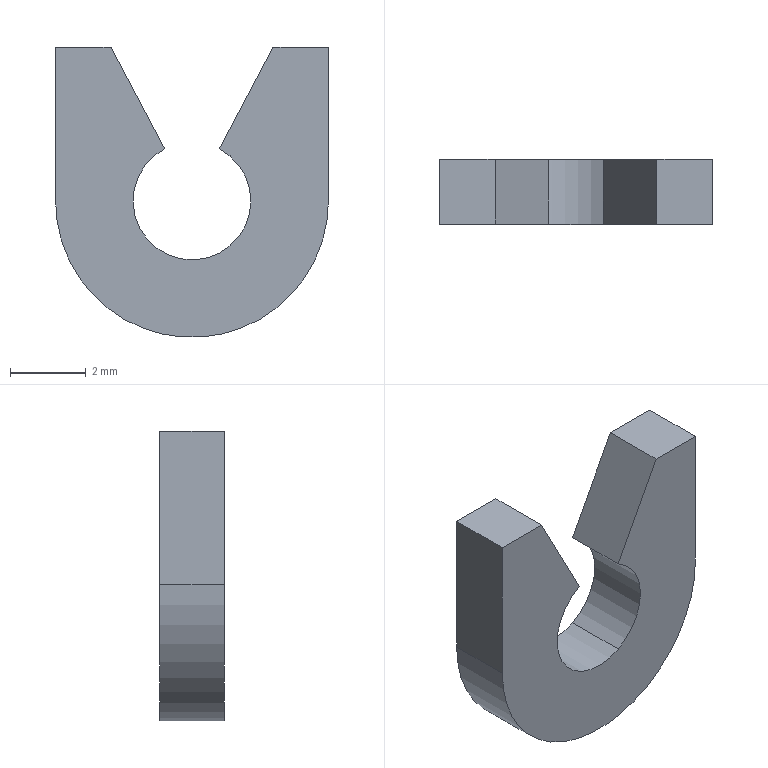Part | SolidWorks | features BaseBody 1 | 1 solid | 11 faces | box 7.18 x 1.7 x 7.64 mm | volume 58.331 mm3 | plane 8 | cylinder 3 | commonest cylinder face diameters 3.1 x2 7.18 x1
STEP:
#1=CARTESIAN_POINT('',(0.7215,1.7,1.372));
#2=VERTEX_POINT('',#1);
#3=CARTESIAN_POINT('',(0.7215,1.7,-1.372));
#4=VERTEX_POINT('',#3);
#5=CARTESIAN_POINT('',(0.,1.7,0.));
#6=DIRECTION('',(0.,1.,0.));
#7=DIRECTION('',(0.4655,0.,0.8851));
#8=AXIS2_PLACEMENT_3D('',#5,#6,#7);
#9=CIRCLE('',#8,1.55);
#10=EDGE_CURVE('',#2,#4,#9,.T.);
#11=ORIENTED_EDGE('',*,*,#10,.T.);
#12=CARTESIAN_POINT('',(0.7215,0.,-1.372));
#13=VERTEX_POINT('',#12);
#14=CARTESIAN_POINT('',(0.7215,1.7,-1.372));
#15=DIRECTION('',(0.,-1.,0.));
#16=VECTOR('',#15,1000.);
#17=LINE('',#14,#16);
#18=EDGE_CURVE('',#4,#13,#17,.T.);
#19=ORIENTED_EDGE('',*,*,#18,.T.);
#20=CARTESIAN_POINT('',(0.7215,0.,1.372));
#21=VERTEX_POINT('',#20);
#22=CARTESIAN_POINT('',(0.,0.,0.));
#23=DIRECTION('',(0.,-1.,0.));
#24=DIRECTION('',(-0.4655,0.,0.8851));
#25=AXIS2_PLACEMENT_3D('',#22,#23,#24);
#26=CIRCLE('',#25,1.55);
#27=EDGE_CURVE('',#13,#21,#26,.T.);
#28=ORIENTED_EDGE('',*,*,#27,.T.);
#29=CARTESIAN_POINT('',(0.7215,0.,1.372));
#30=DIRECTION('',(0.,1.,0.));
#31=VECTOR('',#30,1000.);
#32=LINE('',#29,#31);
#33=EDGE_CURVE('',#21,#2,#32,.T.);
#34=ORIENTED_EDGE('',*,*,#33,.T.);
#35=EDGE_LOOP('',(#11,#19,#28,#34));
#36=FACE_OUTER_BOUND('',#35,.T.);
#37=CARTESIAN_POINT('',(0.,1.7,0.));
#38=DIRECTION('',(0.,-1.,0.));
#39=DIRECTION('',(-0.4655,0.,0.8851));
#40=AXIS2_PLACEMENT_3D('',#37,#38,#39);
#41=CYLINDRICAL_SURFACE('',#40,1.55);
#42=ADVANCED_FACE('',(#36),#41,.F.);
#43=CARTESIAN_POINT('',(-3.59,0.,4.05));
#44=VERTEX_POINT('',#43);
#45=CARTESIAN_POINT('',(-2.13,0.,4.05));
#46=VERTEX_POINT('',#45);
#47=CARTESIAN_POINT('',(-3.59,0.,4.05));
#48=DIRECTION('',(1.,0.,0.));
#49=VECTOR('',#48,1000.);
#50=LINE('',#47,#49);
#51=EDGE_CURVE('',#44,#46,#50,.T.);
#52=ORIENTED_EDGE('',*,*,#51,.F.);
#53=CARTESIAN_POINT('',(-3.59,0.,0.));
#54=VERTEX_POINT('',#53);
#55=CARTESIAN_POINT('',(-3.59,0.,0.));
#56=DIRECTION('',(0.,0.,1.));
#57=VECTOR('',#56,1000.);
#58=LINE('',#55,#57);
#59=EDGE_CURVE('',#54,#44,#58,.T.);
#60=ORIENTED_EDGE('',*,*,#59,.F.);
#61=CARTESIAN_POINT('',(3.59,0.,0.));
#62=VERTEX_POINT('',#61);
#63=CARTESIAN_POINT('',(0.,0.,0.));
#64=DIRECTION('',(0.,1.,0.));
#65=DIRECTION('',(1.,0.,0.));
#66=AXIS2_PLACEMENT_3D('',#63,#64,#65);
#67=CIRCLE('',#66,3.59);
#68=EDGE_CURVE('',#62,#54,#67,.T.);
#69=ORIENTED_EDGE('',*,*,#68,.F.);
#70=CARTESIAN_POINT('',(3.59,0.,4.05));
#71=VERTEX_POINT('',#70);
#72=CARTESIAN_POINT('',(3.59,0.,4.05));
#73=DIRECTION('',(0.,0.,-1.));
#74=VECTOR('',#73,1000.);
#75=LINE('',#72,#74);
#76=EDGE_CURVE('',#71,#62,#75,.T.);
#77=ORIENTED_EDGE('',*,*,#76,.F.);
#78=CARTESIAN_POINT('',(2.13,0.,4.05));
#79=VERTEX_POINT('',#78);
#80=CARTESIAN_POINT('',(2.13,0.,4.05));
#81=DIRECTION('',(1.,0.,0.));
#82=VECTOR('',#81,1000.);
#83=LINE('',#80,#82);
#84=EDGE_CURVE('',#79,#71,#83,.T.);
#85=ORIENTED_EDGE('',*,*,#84,.F.);
#86=CARTESIAN_POINT('',(0.7215,0.,1.372));
#87=DIRECTION('',(0.4655,0.,0.8851));
#88=VECTOR('',#87,1000.);
#89=LINE('',#86,#88);
#90=EDGE_CURVE('',#21,#79,#89,.T.);
#91=ORIENTED_EDGE('',*,*,#90,.F.);
#92=ORIENTED_EDGE('',*,*,#27,.F.);
#93=CARTESIAN_POINT('',(-0.7215,0.,1.372));
#94=VERTEX_POINT('',#93);
#95=CARTESIAN_POINT('',(0.,0.,0.));
#96=DIRECTION('',(0.,-1.,0.));
#97=DIRECTION('',(-0.4655,0.,0.8851));
#98=AXIS2_PLACEMENT_3D('',#95,#96,#97);
#99=CIRCLE('',#98,1.55);
#100=EDGE_CURVE('',#94,#13,#99,.T.);
#101=ORIENTED_EDGE('',*,*,#100,.F.);
#102=CARTESIAN_POINT('',(-2.13,0.,4.05));
#103=DIRECTION('',(0.4655,0.,-0.8851));
#104=VECTOR('',#103,1000.);
#105=LINE('',#102,#104);
#106=EDGE_CURVE('',#46,#94,#105,.T.);
#107=ORIENTED_EDGE('',*,*,#106,.F.);
#108=EDGE_LOOP('',(#52,#60,#69,#77,#85,#91,#92,#101,#107));
#109=FACE_OUTER_BOUND('',#108,.T.);
#110=CARTESIAN_POINT('',(0.,0.,0.));
#111=DIRECTION('',(0.,-1.,0.));
#112=DIRECTION('',(0.,0.,-1.));
#113=AXIS2_PLACEMENT_3D('',#110,#111,#112);
#114=PLANE('',#113);
#115=ADVANCED_FACE('',(#109),#114,.T.);
#116=CARTESIAN_POINT('',(-2.13,1.7,4.05));
#117=VERTEX_POINT('',#116);
#118=CARTESIAN_POINT('',(-3.59,1.7,4.05));
#119=VERTEX_POINT('',#118);
#120=CARTESIAN_POINT('',(-2.13,1.7,4.05));
#121=DIRECTION('',(-1.,0.,0.));
#122=VECTOR('',#121,1000.);
#123=LINE('',#120,#122);
#124=EDGE_CURVE('',#117,#119,#123,.T.);
#125=ORIENTED_EDGE('',*,*,#124,.F.);
#126=CARTESIAN_POINT('',(-0.7215,1.7,1.372));
#127=VERTEX_POINT('',#126);
#128=CARTESIAN_POINT('',(-0.7215,1.7,1.372));
#129=DIRECTION('',(-0.4655,0.,0.8851));
#130=VECTOR('',#129,1000.);
#131=LINE('',#128,#130);
#132=EDGE_CURVE('',#127,#117,#131,.T.);
#133=ORIENTED_EDGE('',*,*,#132,.F.);
#134=CARTESIAN_POINT('',(0.,1.7,0.));
#135=DIRECTION('',(0.,1.,0.));
#136=DIRECTION('',(0.4655,0.,0.8851));
#137=AXIS2_PLACEMENT_3D('',#134,#135,#136);
#138=CIRCLE('',#137,1.55);
#139=EDGE_CURVE('',#4,#127,#138,.T.);
#140=ORIENTED_EDGE('',*,*,#139,.F.);
#141=ORIENTED_EDGE('',*,*,#10,.F.);
#142=CARTESIAN_POINT('',(2.13,1.7,4.05));
#143=VERTEX_POINT('',#142);
#144=CARTESIAN_POINT('',(2.13,1.7,4.05));
#145=DIRECTION('',(-0.4655,0.,-0.8851));
#146=VECTOR('',#145,1000.);
#147=LINE('',#144,#146);
#148=EDGE_CURVE('',#143,#2,#147,.T.);
#149=ORIENTED_EDGE('',*,*,#148,.F.);
#150=CARTESIAN_POINT('',(3.59,1.7,4.05));
#151=VERTEX_POINT('',#150);
#152=CARTESIAN_POINT('',(3.59,1.7,4.05));
#153=DIRECTION('',(-1.,0.,0.));
#154=VECTOR('',#153,1000.);
#155=LINE('',#152,#154);
#156=EDGE_CURVE('',#151,#143,#155,.T.);
#157=ORIENTED_EDGE('',*,*,#156,.F.);
#158=CARTESIAN_POINT('',(3.59,1.7,0.));
#159=VERTEX_POINT('',#158);
#160=CARTESIAN_POINT('',(3.59,1.7,0.));
#161=DIRECTION('',(0.,0.,1.));
#162=VECTOR('',#161,1000.);
#163=LINE('',#160,#162);
#164=EDGE_CURVE('',#159,#151,#163,.T.);
#165=ORIENTED_EDGE('',*,*,#164,.F.);
#166=CARTESIAN_POINT('',(-3.59,1.7,0.));
#167=VERTEX_POINT('',#166);
#168=CARTESIAN_POINT('',(0.,1.7,0.));
#169=DIRECTION('',(0.,-1.,0.));
#170=DIRECTION('',(-1.,0.,0.));
#171=AXIS2_PLACEMENT_3D('',#168,#169,#170);
#172=CIRCLE('',#171,3.59);
#173=EDGE_CURVE('',#167,#159,#172,.T.);
#174=ORIENTED_EDGE('',*,*,#173,.F.);
#175=CARTESIAN_POINT('',(-3.59,1.7,4.05));
#176=DIRECTION('',(0.,0.,-1.));
#177=VECTOR('',#176,1000.);
#178=LINE('',#175,#177);
#179=EDGE_CURVE('',#119,#167,#178,.T.);
#180=ORIENTED_EDGE('',*,*,#179,.F.);
#181=EDGE_LOOP('',(#125,#133,#140,#141,#149,#157,#165,#174,#180));
#182=FACE_OUTER_BOUND('',#181,.T.);
#183=CARTESIAN_POINT('',(0.,1.7,0.));
#184=DIRECTION('',(0.,1.,0.));
#185=DIRECTION('',(1.,0.,0.));
#186=AXIS2_PLACEMENT_3D('',#183,#184,#185);
#187=PLANE('',#186);
#188=ADVANCED_FACE('',(#182),#187,.T.);
#189=ORIENTED_EDGE('',*,*,#59,.T.);
#190=CARTESIAN_POINT('',(-3.59,1.7,4.05));
#191=DIRECTION('',(0.,-1.,0.));
#192=VECTOR('',#191,1000.);
#193=LINE('',#190,#192);
#194=EDGE_CURVE('',#119,#44,#193,.T.);
#195=ORIENTED_EDGE('',*,*,#194,.F.);
#196=ORIENTED_EDGE('',*,*,#179,.T.);
#197=CARTESIAN_POINT('',(-3.59,0.,0.));
#198=DIRECTION('',(0.,1.,0.));
#199=VECTOR('',#198,1000.);
#200=LINE('',#197,#199);
#201=EDGE_CURVE('',#54,#167,#200,.T.);
#202=ORIENTED_EDGE('',*,*,#201,.F.);
#203=EDGE_LOOP('',(#189,#195,#196,#202));
#204=FACE_OUTER_BOUND('',#203,.T.);
#205=CARTESIAN_POINT('',(-3.59,1.7,4.05));
#206=DIRECTION('',(-1.,0.,0.));
#207=DIRECTION('',(0.,0.,1.));
#208=AXIS2_PLACEMENT_3D('',#205,#206,#207);
#209=PLANE('',#208);
#210=ADVANCED_FACE('',(#204),#209,.T.);
#211=ORIENTED_EDGE('',*,*,#68,.T.);
#212=ORIENTED_EDGE('',*,*,#201,.T.);
#213=ORIENTED_EDGE('',*,*,#173,.T.);
#214=CARTESIAN_POINT('',(3.59,0.,0.));
#215=DIRECTION('',(0.,1.,0.));
#216=VECTOR('',#215,1000.);
#217=LINE('',#214,#216);
#218=EDGE_CURVE('',#62,#159,#217,.T.);
#219=ORIENTED_EDGE('',*,*,#218,.F.);
#220=EDGE_LOOP('',(#211,#212,#213,#219));
#221=FACE_OUTER_BOUND('',#220,.T.);
#222=CARTESIAN_POINT('',(0.,1.7,0.));
#223=DIRECTION('',(0.,-1.,0.));
#224=DIRECTION('',(1.,0.,0.));
#225=AXIS2_PLACEMENT_3D('',#222,#223,#224);
#226=CYLINDRICAL_SURFACE('',#225,3.59);
#227=ADVANCED_FACE('',(#221),#226,.T.);
#228=ORIENTED_EDGE('',*,*,#76,.T.);
#229=ORIENTED_EDGE('',*,*,#218,.T.);
#230=ORIENTED_EDGE('',*,*,#164,.T.);
#231=CARTESIAN_POINT('',(3.59,0.,4.05));
#232=DIRECTION('',(0.,1.,0.));
#233=VECTOR('',#232,1000.);
#234=LINE('',#231,#233);
#235=EDGE_CURVE('',#71,#151,#234,.T.);
#236=ORIENTED_EDGE('',*,*,#235,.F.);
#237=EDGE_LOOP('',(#228,#229,#230,#236));
#238=FACE_OUTER_BOUND('',#237,.T.);
#239=CARTESIAN_POINT('',(3.59,1.7,4.05));
#240=DIRECTION('',(1.,0.,0.));
#241=DIRECTION('',(0.,0.,-1.));
#242=AXIS2_PLACEMENT_3D('',#239,#240,#241);
#243=PLANE('',#242);
#244=ADVANCED_FACE('',(#238),#243,.T.);
#245=ORIENTED_EDGE('',*,*,#84,.T.);
#246=ORIENTED_EDGE('',*,*,#235,.T.);
#247=ORIENTED_EDGE('',*,*,#156,.T.);
#248=CARTESIAN_POINT('',(2.13,0.,4.05));
#249=DIRECTION('',(0.,1.,0.));
#250=VECTOR('',#249,1000.);
#251=LINE('',#248,#250);
#252=EDGE_CURVE('',#79,#143,#251,.T.);
#253=ORIENTED_EDGE('',*,*,#252,.F.);
#254=EDGE_LOOP('',(#245,#246,#247,#253));
#255=FACE_OUTER_BOUND('',#254,.T.);
#256=CARTESIAN_POINT('',(2.13,1.7,4.05));
#257=DIRECTION('',(0.,0.,1.));
#258=DIRECTION('',(1.,0.,0.));
#259=AXIS2_PLACEMENT_3D('',#256,#257,#258);
#260=PLANE('',#259);
#261=ADVANCED_FACE('',(#255),#260,.T.);
#262=ORIENTED_EDGE('',*,*,#90,.T.);
#263=ORIENTED_EDGE('',*,*,#252,.T.);
#264=ORIENTED_EDGE('',*,*,#148,.T.);
#265=ORIENTED_EDGE('',*,*,#33,.F.);
#266=EDGE_LOOP('',(#262,#263,#264,#265));
#267=FACE_OUTER_BOUND('',#266,.T.);
#268=CARTESIAN_POINT('',(0.7215,1.7,1.372));
#269=DIRECTION('',(-0.8851,0.,0.4655));
#270=DIRECTION('',(0.,1.,0.));
#271=AXIS2_PLACEMENT_3D('',#268,#269,#270);
#272=PLANE('',#271);
#273=ADVANCED_FACE('',(#267),#272,.T.);
#274=ORIENTED_EDGE('',*,*,#18,.F.);
#275=ORIENTED_EDGE('',*,*,#139,.T.);
#276=CARTESIAN_POINT('',(-0.7215,0.,1.372));
#277=DIRECTION('',(0.,1.,0.));
#278=VECTOR('',#277,1000.);
#279=LINE('',#276,#278);
#280=EDGE_CURVE('',#94,#127,#279,.T.);
#281=ORIENTED_EDGE('',*,*,#280,.F.);
#282=ORIENTED_EDGE('',*,*,#100,.T.);
#283=EDGE_LOOP('',(#274,#275,#281,#282));
#284=FACE_OUTER_BOUND('',#283,.T.);
#285=CARTESIAN_POINT('',(0.,1.7,0.));
#286=DIRECTION('',(0.,-1.,0.));
#287=DIRECTION('',(-0.4655,0.,0.8851));
#288=AXIS2_PLACEMENT_3D('',#285,#286,#287);
#289=CYLINDRICAL_SURFACE('',#288,1.55);
#290=ADVANCED_FACE('',(#284),#289,.F.);
#291=ORIENTED_EDGE('',*,*,#106,.T.);
#292=ORIENTED_EDGE('',*,*,#280,.T.);
#293=ORIENTED_EDGE('',*,*,#132,.T.);
#294=CARTESIAN_POINT('',(-2.13,0.,4.05));
#295=DIRECTION('',(0.,1.,0.));
#296=VECTOR('',#295,1000.);
#297=LINE('',#294,#296);
#298=EDGE_CURVE('',#46,#117,#297,.T.);
#299=ORIENTED_EDGE('',*,*,#298,.F.);
#300=EDGE_LOOP('',(#291,#292,#293,#299));
#301=FACE_OUTER_BOUND('',#300,.T.);
#302=CARTESIAN_POINT('',(-0.7215,1.7,1.372));
#303=DIRECTION('',(0.8851,0.,0.4655));
#304=DIRECTION('',(0.,-1.,0.));
#305=AXIS2_PLACEMENT_3D('',#302,#303,#304);
#306=PLANE('',#305);
#307=ADVANCED_FACE('',(#301),#306,.T.);
#308=ORIENTED_EDGE('',*,*,#51,.T.);
#309=ORIENTED_EDGE('',*,*,#298,.T.);
#310=ORIENTED_EDGE('',*,*,#124,.T.);
#311=ORIENTED_EDGE('',*,*,#194,.T.);
#312=EDGE_LOOP('',(#308,#309,#310,#311));
#313=FACE_OUTER_BOUND('',#312,.T.);
#314=CARTESIAN_POINT('',(-2.13,1.7,4.05));
#315=DIRECTION('',(0.,0.,1.));
#316=DIRECTION('',(1.,0.,0.));
#317=AXIS2_PLACEMENT_3D('',#314,#315,#316);
#318=PLANE('',#317);
#319=ADVANCED_FACE('',(#313),#318,.T.);
#320=CLOSED_SHELL('',(#42,#115,#188,#210,#227,#244,#261,#273,#290,#307,#319));
#321=MANIFOLD_SOLID_BREP('',#320);
#322=CARTESIAN_POINT('',(0.,0.,0.));
#323=DIRECTION('',(0.,0.,1.));
#324=DIRECTION('',(1.,0.,0.));
#325=AXIS2_PLACEMENT_3D('',#322,#323,#324);
#326=(LENGTH_UNIT()NAMED_UNIT(*)SI_UNIT(.MILLI.,.METRE.));
#327=UNCERTAINTY_MEASURE_WITH_UNIT(LENGTH_MEASURE(0.00001),#326,'','');
#328=(NAMED_UNIT(*)PLANE_ANGLE_UNIT()SI_UNIT($,.RADIAN.));
#329=(NAMED_UNIT(*)SI_UNIT($,.STERADIAN.)SOLID_ANGLE_UNIT());
#330=(GEOMETRIC_REPRESENTATION_CONTEXT(3)GLOBAL_UNCERTAINTY_ASSIGNED_CONTEXT((#327))GLOBAL_UNIT_ASSIGNED_CONTEXT((#326,#328,#329))REPRESENTATION_CONTEXT('',''));
#331=ADVANCED_BREP_SHAPE_REPRESENTATION('',(#321,#325),#330);